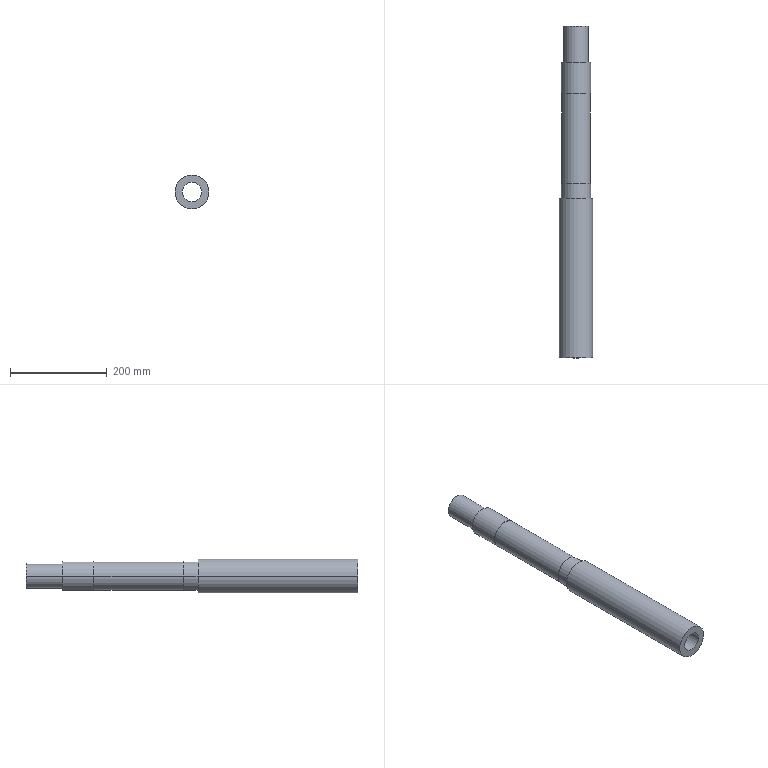Part | SolidWorks | features ICE 1, Revolution 1 | 1 solid | 18 faces | box 70 x 685 x 70 mm | volume 1330845 mm3 | cylinder 12 | plane 6 | commonest cylinder face diameters 60 x4 40 x2 50 x2 59 x2 70 x2
STEP:
#1=CARTESIAN_POINT('',(-20.,0.,0.));
#2=VERTEX_POINT('',#1);
#3=CARTESIAN_POINT('',(20.,0.,0.));
#4=VERTEX_POINT('',#3);
#5=CARTESIAN_POINT('',(0.,0.,0.));
#6=DIRECTION('',(0.,-1.,0.));
#7=DIRECTION('',(-1.,0.,0.));
#8=AXIS2_PLACEMENT_3D('',#5,#6,#7);
#9=CIRCLE('',#8,20.);
#10=EDGE_CURVE('',#2,#4,#9,.T.);
#11=ORIENTED_EDGE('',*,*,#10,.T.);
#12=CARTESIAN_POINT('',(20.,685.,0.));
#13=VERTEX_POINT('',#12);
#14=CARTESIAN_POINT('',(20.,-0.001,0.));
#15=DIRECTION('',(0.,1.,0.));
#16=VECTOR('',#15,1000.);
#17=LINE('',#14,#16);
#18=EDGE_CURVE('',#4,#13,#17,.T.);
#19=ORIENTED_EDGE('',*,*,#18,.T.);
#20=CARTESIAN_POINT('',(-20.,685.,0.));
#21=VERTEX_POINT('',#20);
#22=CARTESIAN_POINT('',(0.,685.,0.));
#23=DIRECTION('',(0.,1.,0.));
#24=DIRECTION('',(-1.,0.,0.));
#25=AXIS2_PLACEMENT_3D('',#22,#23,#24);
#26=CIRCLE('',#25,20.);
#27=EDGE_CURVE('',#13,#21,#26,.T.);
#28=ORIENTED_EDGE('',*,*,#27,.T.);
#29=CARTESIAN_POINT('',(-20.,-0.001,0.));
#30=DIRECTION('',(0.,1.,0.));
#31=VECTOR('',#30,1000.);
#32=LINE('',#29,#31);
#33=EDGE_CURVE('',#2,#21,#32,.T.);
#34=ORIENTED_EDGE('',*,*,#33,.F.);
#35=EDGE_LOOP('',(#11,#19,#28,#34));
#36=FACE_OUTER_BOUND('',#35,.T.);
#37=CARTESIAN_POINT('',(0.,-0.001,0.));
#38=DIRECTION('',(0.,1.,0.));
#39=DIRECTION('',(-1.,0.,0.));
#40=AXIS2_PLACEMENT_3D('',#37,#38,#39);
#41=CYLINDRICAL_SURFACE('',#40,20.);
#42=ADVANCED_FACE('',(#36),#41,.F.);
#43=CARTESIAN_POINT('',(-25.,610.,0.));
#44=VERTEX_POINT('',#43);
#45=CARTESIAN_POINT('',(25.,610.,0.));
#46=VERTEX_POINT('',#45);
#47=CARTESIAN_POINT('',(0.,610.,0.));
#48=DIRECTION('',(0.,1.,0.));
#49=DIRECTION('',(-1.,0.,0.));
#50=AXIS2_PLACEMENT_3D('',#47,#48,#49);
#51=CIRCLE('',#50,25.);
#52=EDGE_CURVE('',#44,#46,#51,.T.);
#53=ORIENTED_EDGE('',*,*,#52,.T.);
#54=CARTESIAN_POINT('',(25.,685.,0.));
#55=VERTEX_POINT('',#54);
#56=CARTESIAN_POINT('',(25.,685.,0.));
#57=DIRECTION('',(0.,1.,0.));
#58=VECTOR('',#57,1000.);
#59=LINE('',#56,#58);
#60=EDGE_CURVE('',#46,#55,#59,.T.);
#61=ORIENTED_EDGE('',*,*,#60,.T.);
#62=CARTESIAN_POINT('',(-25.,685.,0.));
#63=VERTEX_POINT('',#62);
#64=CARTESIAN_POINT('',(0.,685.,0.));
#65=DIRECTION('',(0.,1.,0.));
#66=DIRECTION('',(-1.,0.,0.));
#67=AXIS2_PLACEMENT_3D('',#64,#65,#66);
#68=CIRCLE('',#67,25.);
#69=EDGE_CURVE('',#63,#55,#68,.T.);
#70=ORIENTED_EDGE('',*,*,#69,.F.);
#71=CARTESIAN_POINT('',(-25.,685.,0.));
#72=DIRECTION('',(0.,1.,0.));
#73=VECTOR('',#72,1000.);
#74=LINE('',#71,#73);
#75=EDGE_CURVE('',#44,#63,#74,.T.);
#76=ORIENTED_EDGE('',*,*,#75,.F.);
#77=EDGE_LOOP('',(#53,#61,#70,#76));
#78=FACE_OUTER_BOUND('',#77,.T.);
#79=CARTESIAN_POINT('',(0.,685.,0.));
#80=DIRECTION('',(0.,1.,0.));
#81=DIRECTION('',(-1.,0.,0.));
#82=AXIS2_PLACEMENT_3D('',#79,#80,#81);
#83=CYLINDRICAL_SURFACE('',#82,25.);
#84=ADVANCED_FACE('',(#78),#83,.T.);
#85=CARTESIAN_POINT('',(-30.,545.,0.));
#86=VERTEX_POINT('',#85);
#87=CARTESIAN_POINT('',(30.,545.,0.));
#88=VERTEX_POINT('',#87);
#89=CARTESIAN_POINT('',(0.,545.,0.));
#90=DIRECTION('',(0.,1.,0.));
#91=DIRECTION('',(-1.,0.,0.));
#92=AXIS2_PLACEMENT_3D('',#89,#90,#91);
#93=CIRCLE('',#92,30.);
#94=EDGE_CURVE('',#86,#88,#93,.T.);
#95=ORIENTED_EDGE('',*,*,#94,.T.);
#96=CARTESIAN_POINT('',(30.,610.,0.));
#97=VERTEX_POINT('',#96);
#98=CARTESIAN_POINT('',(30.,685.,0.));
#99=DIRECTION('',(0.,1.,0.));
#100=VECTOR('',#99,1000.);
#101=LINE('',#98,#100);
#102=EDGE_CURVE('',#88,#97,#101,.T.);
#103=ORIENTED_EDGE('',*,*,#102,.T.);
#104=CARTESIAN_POINT('',(-30.,610.,0.));
#105=VERTEX_POINT('',#104);
#106=CARTESIAN_POINT('',(0.,610.,0.));
#107=DIRECTION('',(0.,1.,0.));
#108=DIRECTION('',(-1.,0.,0.));
#109=AXIS2_PLACEMENT_3D('',#106,#107,#108);
#110=CIRCLE('',#109,30.);
#111=EDGE_CURVE('',#105,#97,#110,.T.);
#112=ORIENTED_EDGE('',*,*,#111,.F.);
#113=CARTESIAN_POINT('',(-30.,685.,0.));
#114=DIRECTION('',(0.,1.,0.));
#115=VECTOR('',#114,1000.);
#116=LINE('',#113,#115);
#117=EDGE_CURVE('',#86,#105,#116,.T.);
#118=ORIENTED_EDGE('',*,*,#117,.F.);
#119=EDGE_LOOP('',(#95,#103,#112,#118));
#120=FACE_OUTER_BOUND('',#119,.T.);
#121=CARTESIAN_POINT('',(0.,685.,0.));
#122=DIRECTION('',(0.,1.,0.));
#123=DIRECTION('',(-1.,0.,0.));
#124=AXIS2_PLACEMENT_3D('',#121,#122,#123);
#125=CYLINDRICAL_SURFACE('',#124,30.);
#126=ADVANCED_FACE('',(#120),#125,.T.);
#127=CARTESIAN_POINT('',(-29.5,360.,0.));
#128=VERTEX_POINT('',#127);
#129=CARTESIAN_POINT('',(29.5,360.,0.));
#130=VERTEX_POINT('',#129);
#131=CARTESIAN_POINT('',(0.,360.,0.));
#132=DIRECTION('',(0.,1.,0.));
#133=DIRECTION('',(-1.,0.,0.));
#134=AXIS2_PLACEMENT_3D('',#131,#132,#133);
#135=CIRCLE('',#134,29.5);
#136=EDGE_CURVE('',#128,#130,#135,.T.);
#137=ORIENTED_EDGE('',*,*,#136,.T.);
#138=CARTESIAN_POINT('',(29.5,545.,0.));
#139=VERTEX_POINT('',#138);
#140=CARTESIAN_POINT('',(29.5,685.,0.));
#141=DIRECTION('',(0.,1.,0.));
#142=VECTOR('',#141,1000.);
#143=LINE('',#140,#142);
#144=EDGE_CURVE('',#130,#139,#143,.T.);
#145=ORIENTED_EDGE('',*,*,#144,.T.);
#146=CARTESIAN_POINT('',(-29.5,545.,0.));
#147=VERTEX_POINT('',#146);
#148=CARTESIAN_POINT('',(0.,545.,0.));
#149=DIRECTION('',(0.,1.,0.));
#150=DIRECTION('',(-1.,0.,0.));
#151=AXIS2_PLACEMENT_3D('',#148,#149,#150);
#152=CIRCLE('',#151,29.5);
#153=EDGE_CURVE('',#147,#139,#152,.T.);
#154=ORIENTED_EDGE('',*,*,#153,.F.);
#155=CARTESIAN_POINT('',(-29.5,685.,0.));
#156=DIRECTION('',(0.,1.,0.));
#157=VECTOR('',#156,1000.);
#158=LINE('',#155,#157);
#159=EDGE_CURVE('',#128,#147,#158,.T.);
#160=ORIENTED_EDGE('',*,*,#159,.F.);
#161=EDGE_LOOP('',(#137,#145,#154,#160));
#162=FACE_OUTER_BOUND('',#161,.T.);
#163=CARTESIAN_POINT('',(0.,685.,0.));
#164=DIRECTION('',(0.,1.,0.));
#165=DIRECTION('',(-1.,0.,0.));
#166=AXIS2_PLACEMENT_3D('',#163,#164,#165);
#167=CYLINDRICAL_SURFACE('',#166,29.5);
#168=ADVANCED_FACE('',(#162),#167,.T.);
#169=CARTESIAN_POINT('',(-30.,330.,0.));
#170=VERTEX_POINT('',#169);
#171=CARTESIAN_POINT('',(30.,330.,0.));
#172=VERTEX_POINT('',#171);
#173=CARTESIAN_POINT('',(0.,330.,0.));
#174=DIRECTION('',(0.,1.,0.));
#175=DIRECTION('',(-1.,0.,0.));
#176=AXIS2_PLACEMENT_3D('',#173,#174,#175);
#177=CIRCLE('',#176,30.);
#178=EDGE_CURVE('',#170,#172,#177,.T.);
#179=ORIENTED_EDGE('',*,*,#178,.T.);
#180=CARTESIAN_POINT('',(30.,360.,0.));
#181=VERTEX_POINT('',#180);
#182=CARTESIAN_POINT('',(30.,685.,0.));
#183=DIRECTION('',(0.,1.,0.));
#184=VECTOR('',#183,1000.);
#185=LINE('',#182,#184);
#186=EDGE_CURVE('',#172,#181,#185,.T.);
#187=ORIENTED_EDGE('',*,*,#186,.T.);
#188=CARTESIAN_POINT('',(-30.,360.,0.));
#189=VERTEX_POINT('',#188);
#190=CARTESIAN_POINT('',(0.,360.,0.));
#191=DIRECTION('',(0.,1.,0.));
#192=DIRECTION('',(-1.,0.,0.));
#193=AXIS2_PLACEMENT_3D('',#190,#191,#192);
#194=CIRCLE('',#193,30.);
#195=EDGE_CURVE('',#189,#181,#194,.T.);
#196=ORIENTED_EDGE('',*,*,#195,.F.);
#197=CARTESIAN_POINT('',(-30.,685.,0.));
#198=DIRECTION('',(0.,1.,0.));
#199=VECTOR('',#198,1000.);
#200=LINE('',#197,#199);
#201=EDGE_CURVE('',#170,#189,#200,.T.);
#202=ORIENTED_EDGE('',*,*,#201,.F.);
#203=EDGE_LOOP('',(#179,#187,#196,#202));
#204=FACE_OUTER_BOUND('',#203,.T.);
#205=CARTESIAN_POINT('',(0.,685.,0.));
#206=DIRECTION('',(0.,1.,0.));
#207=DIRECTION('',(-1.,0.,0.));
#208=AXIS2_PLACEMENT_3D('',#205,#206,#207);
#209=CYLINDRICAL_SURFACE('',#208,30.);
#210=ADVANCED_FACE('',(#204),#209,.T.);
#211=CARTESIAN_POINT('',(-35.,0.,0.));
#212=VERTEX_POINT('',#211);
#213=CARTESIAN_POINT('',(35.,0.,0.));
#214=VERTEX_POINT('',#213);
#215=CARTESIAN_POINT('',(0.,0.,0.));
#216=DIRECTION('',(0.,1.,0.));
#217=DIRECTION('',(-1.,0.,0.));
#218=AXIS2_PLACEMENT_3D('',#215,#216,#217);
#219=CIRCLE('',#218,35.);
#220=EDGE_CURVE('',#212,#214,#219,.T.);
#221=ORIENTED_EDGE('',*,*,#220,.T.);
#222=CARTESIAN_POINT('',(35.,330.,0.));
#223=VERTEX_POINT('',#222);
#224=CARTESIAN_POINT('',(35.,685.,0.));
#225=DIRECTION('',(0.,1.,0.));
#226=VECTOR('',#225,1000.);
#227=LINE('',#224,#226);
#228=EDGE_CURVE('',#214,#223,#227,.T.);
#229=ORIENTED_EDGE('',*,*,#228,.T.);
#230=CARTESIAN_POINT('',(-35.,330.,0.));
#231=VERTEX_POINT('',#230);
#232=CARTESIAN_POINT('',(0.,330.,0.));
#233=DIRECTION('',(0.,1.,0.));
#234=DIRECTION('',(-1.,0.,0.));
#235=AXIS2_PLACEMENT_3D('',#232,#233,#234);
#236=CIRCLE('',#235,35.);
#237=EDGE_CURVE('',#231,#223,#236,.T.);
#238=ORIENTED_EDGE('',*,*,#237,.F.);
#239=CARTESIAN_POINT('',(-35.,685.,0.));
#240=DIRECTION('',(0.,1.,0.));
#241=VECTOR('',#240,1000.);
#242=LINE('',#239,#241);
#243=EDGE_CURVE('',#212,#231,#242,.T.);
#244=ORIENTED_EDGE('',*,*,#243,.F.);
#245=EDGE_LOOP('',(#221,#229,#238,#244));
#246=FACE_OUTER_BOUND('',#245,.T.);
#247=CARTESIAN_POINT('',(0.,685.,0.));
#248=DIRECTION('',(0.,1.,0.));
#249=DIRECTION('',(-1.,0.,0.));
#250=AXIS2_PLACEMENT_3D('',#247,#248,#249);
#251=CYLINDRICAL_SURFACE('',#250,35.);
#252=ADVANCED_FACE('',(#246),#251,.T.);
#253=ORIENTED_EDGE('',*,*,#10,.F.);
#254=CARTESIAN_POINT('',(0.,0.,0.));
#255=DIRECTION('',(0.,-1.,0.));
#256=DIRECTION('',(-1.,0.,0.));
#257=AXIS2_PLACEMENT_3D('',#254,#255,#256);
#258=CIRCLE('',#257,20.);
#259=EDGE_CURVE('',#4,#2,#258,.T.);
#260=ORIENTED_EDGE('',*,*,#259,.F.);
#261=EDGE_LOOP('',(#253,#260));
#262=FACE_BOUND('',#261,.T.);
#263=ORIENTED_EDGE('',*,*,#220,.F.);
#264=CARTESIAN_POINT('',(0.,0.,0.));
#265=DIRECTION('',(0.,1.,0.));
#266=DIRECTION('',(-1.,0.,0.));
#267=AXIS2_PLACEMENT_3D('',#264,#265,#266);
#268=CIRCLE('',#267,35.);
#269=EDGE_CURVE('',#214,#212,#268,.T.);
#270=ORIENTED_EDGE('',*,*,#269,.F.);
#271=EDGE_LOOP('',(#263,#270));
#272=FACE_OUTER_BOUND('',#271,.T.);
#273=CARTESIAN_POINT('',(0.,0.,0.));
#274=DIRECTION('',(0.,1.,0.));
#275=DIRECTION('',(-1.,0.,0.));
#276=AXIS2_PLACEMENT_3D('',#273,#274,#275);
#277=PLANE('',#276);
#278=ADVANCED_FACE('',(#262,#272),#277,.F.);
#279=ORIENTED_EDGE('',*,*,#228,.F.);
#280=ORIENTED_EDGE('',*,*,#269,.T.);
#281=ORIENTED_EDGE('',*,*,#243,.T.);
#282=CARTESIAN_POINT('',(0.,330.,0.));
#283=DIRECTION('',(0.,1.,0.));
#284=DIRECTION('',(-1.,0.,0.));
#285=AXIS2_PLACEMENT_3D('',#282,#283,#284);
#286=CIRCLE('',#285,35.);
#287=EDGE_CURVE('',#223,#231,#286,.T.);
#288=ORIENTED_EDGE('',*,*,#287,.F.);
#289=EDGE_LOOP('',(#279,#280,#281,#288));
#290=FACE_OUTER_BOUND('',#289,.T.);
#291=CARTESIAN_POINT('',(0.,685.,0.));
#292=DIRECTION('',(0.,1.,0.));
#293=DIRECTION('',(-1.,0.,0.));
#294=AXIS2_PLACEMENT_3D('',#291,#292,#293);
#295=CYLINDRICAL_SURFACE('',#294,35.);
#296=ADVANCED_FACE('',(#290),#295,.T.);
#297=ORIENTED_EDGE('',*,*,#178,.F.);
#298=CARTESIAN_POINT('',(0.,330.,0.));
#299=DIRECTION('',(0.,1.,0.));
#300=DIRECTION('',(-1.,0.,0.));
#301=AXIS2_PLACEMENT_3D('',#298,#299,#300);
#302=CIRCLE('',#301,30.);
#303=EDGE_CURVE('',#172,#170,#302,.T.);
#304=ORIENTED_EDGE('',*,*,#303,.F.);
#305=EDGE_LOOP('',(#297,#304));
#306=FACE_BOUND('',#305,.T.);
#307=ORIENTED_EDGE('',*,*,#237,.T.);
#308=ORIENTED_EDGE('',*,*,#287,.T.);
#309=EDGE_LOOP('',(#307,#308));
#310=FACE_OUTER_BOUND('',#309,.T.);
#311=CARTESIAN_POINT('',(35.,330.,0.));
#312=DIRECTION('',(0.,-1.,0.));
#313=DIRECTION('',(1.,0.,0.));
#314=AXIS2_PLACEMENT_3D('',#311,#312,#313);
#315=PLANE('',#314);
#316=ADVANCED_FACE('',(#306,#310),#315,.F.);
#317=ORIENTED_EDGE('',*,*,#186,.F.);
#318=ORIENTED_EDGE('',*,*,#303,.T.);
#319=ORIENTED_EDGE('',*,*,#201,.T.);
#320=CARTESIAN_POINT('',(0.,360.,0.));
#321=DIRECTION('',(0.,1.,0.));
#322=DIRECTION('',(-1.,0.,0.));
#323=AXIS2_PLACEMENT_3D('',#320,#321,#322);
#324=CIRCLE('',#323,30.);
#325=EDGE_CURVE('',#181,#189,#324,.T.);
#326=ORIENTED_EDGE('',*,*,#325,.F.);
#327=EDGE_LOOP('',(#317,#318,#319,#326));
#328=FACE_OUTER_BOUND('',#327,.T.);
#329=CARTESIAN_POINT('',(0.,685.,0.));
#330=DIRECTION('',(0.,1.,0.));
#331=DIRECTION('',(-1.,0.,0.));
#332=AXIS2_PLACEMENT_3D('',#329,#330,#331);
#333=CYLINDRICAL_SURFACE('',#332,30.);
#334=ADVANCED_FACE('',(#328),#333,.T.);
#335=ORIENTED_EDGE('',*,*,#136,.F.);
#336=CARTESIAN_POINT('',(0.,360.,0.));
#337=DIRECTION('',(0.,1.,0.));
#338=DIRECTION('',(-1.,0.,0.));
#339=AXIS2_PLACEMENT_3D('',#336,#337,#338);
#340=CIRCLE('',#339,29.5);
#341=EDGE_CURVE('',#130,#128,#340,.T.);
#342=ORIENTED_EDGE('',*,*,#341,.F.);
#343=EDGE_LOOP('',(#335,#342));
#344=FACE_BOUND('',#343,.T.);
#345=ORIENTED_EDGE('',*,*,#195,.T.);
#346=ORIENTED_EDGE('',*,*,#325,.T.);
#347=EDGE_LOOP('',(#345,#346));
#348=FACE_OUTER_BOUND('',#347,.T.);
#349=CARTESIAN_POINT('',(30.,360.,0.));
#350=DIRECTION('',(0.,-1.,0.));
#351=DIRECTION('',(1.,0.,0.));
#352=AXIS2_PLACEMENT_3D('',#349,#350,#351);
#353=PLANE('',#352);
#354=ADVANCED_FACE('',(#344,#348),#353,.F.);
#355=ORIENTED_EDGE('',*,*,#144,.F.);
#356=ORIENTED_EDGE('',*,*,#341,.T.);
#357=ORIENTED_EDGE('',*,*,#159,.T.);
#358=CARTESIAN_POINT('',(0.,545.,0.));
#359=DIRECTION('',(0.,1.,0.));
#360=DIRECTION('',(-1.,0.,0.));
#361=AXIS2_PLACEMENT_3D('',#358,#359,#360);
#362=CIRCLE('',#361,29.5);
#363=EDGE_CURVE('',#139,#147,#362,.T.);
#364=ORIENTED_EDGE('',*,*,#363,.F.);
#365=EDGE_LOOP('',(#355,#356,#357,#364));
#366=FACE_OUTER_BOUND('',#365,.T.);
#367=CARTESIAN_POINT('',(0.,685.,0.));
#368=DIRECTION('',(0.,1.,0.));
#369=DIRECTION('',(-1.,0.,0.));
#370=AXIS2_PLACEMENT_3D('',#367,#368,#369);
#371=CYLINDRICAL_SURFACE('',#370,29.5);
#372=ADVANCED_FACE('',(#366),#371,.T.);
#373=ORIENTED_EDGE('',*,*,#94,.F.);
#374=CARTESIAN_POINT('',(0.,545.,0.));
#375=DIRECTION('',(0.,1.,0.));
#376=DIRECTION('',(-1.,0.,0.));
#377=AXIS2_PLACEMENT_3D('',#374,#375,#376);
#378=CIRCLE('',#377,30.);
#379=EDGE_CURVE('',#88,#86,#378,.T.);
#380=ORIENTED_EDGE('',*,*,#379,.F.);
#381=EDGE_LOOP('',(#373,#380));
#382=FACE_OUTER_BOUND('',#381,.T.);
#383=ORIENTED_EDGE('',*,*,#153,.T.);
#384=ORIENTED_EDGE('',*,*,#363,.T.);
#385=EDGE_LOOP('',(#383,#384));
#386=FACE_BOUND('',#385,.T.);
#387=CARTESIAN_POINT('',(29.5,545.,0.));
#388=DIRECTION('',(0.,1.,0.));
#389=DIRECTION('',(-1.,0.,0.));
#390=AXIS2_PLACEMENT_3D('',#387,#388,#389);
#391=PLANE('',#390);
#392=ADVANCED_FACE('',(#382,#386),#391,.F.);
#393=ORIENTED_EDGE('',*,*,#102,.F.);
#394=ORIENTED_EDGE('',*,*,#379,.T.);
#395=ORIENTED_EDGE('',*,*,#117,.T.);
#396=CARTESIAN_POINT('',(0.,610.,0.));
#397=DIRECTION('',(0.,1.,0.));
#398=DIRECTION('',(-1.,0.,0.));
#399=AXIS2_PLACEMENT_3D('',#396,#397,#398);
#400=CIRCLE('',#399,30.);
#401=EDGE_CURVE('',#97,#105,#400,.T.);
#402=ORIENTED_EDGE('',*,*,#401,.F.);
#403=EDGE_LOOP('',(#393,#394,#395,#402));
#404=FACE_OUTER_BOUND('',#403,.T.);
#405=CARTESIAN_POINT('',(0.,685.,0.));
#406=DIRECTION('',(0.,1.,0.));
#407=DIRECTION('',(-1.,0.,0.));
#408=AXIS2_PLACEMENT_3D('',#405,#406,#407);
#409=CYLINDRICAL_SURFACE('',#408,30.);
#410=ADVANCED_FACE('',(#404),#409,.T.);
#411=ORIENTED_EDGE('',*,*,#52,.F.);
#412=CARTESIAN_POINT('',(0.,610.,0.));
#413=DIRECTION('',(0.,1.,0.));
#414=DIRECTION('',(-1.,0.,0.));
#415=AXIS2_PLACEMENT_3D('',#412,#413,#414);
#416=CIRCLE('',#415,25.);
#417=EDGE_CURVE('',#46,#44,#416,.T.);
#418=ORIENTED_EDGE('',*,*,#417,.F.);
#419=EDGE_LOOP('',(#411,#418));
#420=FACE_BOUND('',#419,.T.);
#421=ORIENTED_EDGE('',*,*,#111,.T.);
#422=ORIENTED_EDGE('',*,*,#401,.T.);
#423=EDGE_LOOP('',(#421,#422));
#424=FACE_OUTER_BOUND('',#423,.T.);
#425=CARTESIAN_POINT('',(30.,610.,0.));
#426=DIRECTION('',(0.,-1.,0.));
#427=DIRECTION('',(1.,0.,0.));
#428=AXIS2_PLACEMENT_3D('',#425,#426,#427);
#429=PLANE('',#428);
#430=ADVANCED_FACE('',(#420,#424),#429,.F.);
#431=ORIENTED_EDGE('',*,*,#60,.F.);
#432=ORIENTED_EDGE('',*,*,#417,.T.);
#433=ORIENTED_EDGE('',*,*,#75,.T.);
#434=CARTESIAN_POINT('',(0.,685.,0.));
#435=DIRECTION('',(0.,1.,0.));
#436=DIRECTION('',(-1.,0.,0.));
#437=AXIS2_PLACEMENT_3D('',#434,#435,#436);
#438=CIRCLE('',#437,25.);
#439=EDGE_CURVE('',#55,#63,#438,.T.);
#440=ORIENTED_EDGE('',*,*,#439,.F.);
#441=EDGE_LOOP('',(#431,#432,#433,#440));
#442=FACE_OUTER_BOUND('',#441,.T.);
#443=CARTESIAN_POINT('',(0.,685.,0.));
#444=DIRECTION('',(0.,1.,0.));
#445=DIRECTION('',(-1.,0.,0.));
#446=AXIS2_PLACEMENT_3D('',#443,#444,#445);
#447=CYLINDRICAL_SURFACE('',#446,25.);
#448=ADVANCED_FACE('',(#442),#447,.T.);
#449=CARTESIAN_POINT('',(0.,685.,0.));
#450=DIRECTION('',(0.,1.,0.));
#451=DIRECTION('',(-1.,0.,0.));
#452=AXIS2_PLACEMENT_3D('',#449,#450,#451);
#453=CIRCLE('',#452,20.);
#454=EDGE_CURVE('',#21,#13,#453,.T.);
#455=ORIENTED_EDGE('',*,*,#454,.F.);
#456=ORIENTED_EDGE('',*,*,#27,.F.);
#457=EDGE_LOOP('',(#455,#456));
#458=FACE_BOUND('',#457,.T.);
#459=ORIENTED_EDGE('',*,*,#69,.T.);
#460=ORIENTED_EDGE('',*,*,#439,.T.);
#461=EDGE_LOOP('',(#459,#460));
#462=FACE_OUTER_BOUND('',#461,.T.);
#463=CARTESIAN_POINT('',(25.,685.,0.));
#464=DIRECTION('',(0.,-1.,0.));
#465=DIRECTION('',(1.,0.,0.));
#466=AXIS2_PLACEMENT_3D('',#463,#464,#465);
#467=PLANE('',#466);
#468=ADVANCED_FACE('',(#458,#462),#467,.F.);
#469=ORIENTED_EDGE('',*,*,#18,.F.);
#470=ORIENTED_EDGE('',*,*,#259,.T.);
#471=ORIENTED_EDGE('',*,*,#33,.T.);
#472=ORIENTED_EDGE('',*,*,#454,.T.);
#473=EDGE_LOOP('',(#469,#470,#471,#472));
#474=FACE_OUTER_BOUND('',#473,.T.);
#475=CARTESIAN_POINT('',(0.,-0.001,0.));
#476=DIRECTION('',(0.,1.,0.));
#477=DIRECTION('',(-1.,0.,0.));
#478=AXIS2_PLACEMENT_3D('',#475,#476,#477);
#479=CYLINDRICAL_SURFACE('',#478,20.);
#480=ADVANCED_FACE('',(#474),#479,.F.);
#481=CLOSED_SHELL('',(#42,#84,#126,#168,#210,#252,#278,#296,#316,#334,#354,#372,#392,#410,#430,#448,#468,#480));
#482=MANIFOLD_SOLID_BREP('',#481);
#483=CARTESIAN_POINT('',(0.,0.,0.));
#484=DIRECTION('',(0.,0.,1.));
#485=DIRECTION('',(1.,0.,0.));
#486=AXIS2_PLACEMENT_3D('',#483,#484,#485);
#487=(LENGTH_UNIT()NAMED_UNIT(*)SI_UNIT(.MILLI.,.METRE.));
#488=UNCERTAINTY_MEASURE_WITH_UNIT(LENGTH_MEASURE(0.00001),#487,'','');
#489=(NAMED_UNIT(*)PLANE_ANGLE_UNIT()SI_UNIT($,.RADIAN.));
#490=(NAMED_UNIT(*)SI_UNIT($,.STERADIAN.)SOLID_ANGLE_UNIT());
#491=(GEOMETRIC_REPRESENTATION_CONTEXT(3)GLOBAL_UNCERTAINTY_ASSIGNED_CONTEXT((#488))GLOBAL_UNIT_ASSIGNED_CONTEXT((#487,#489,#490))REPRESENTATION_CONTEXT('',''));
#492=ADVANCED_BREP_SHAPE_REPRESENTATION('',(#482,#486),#491);